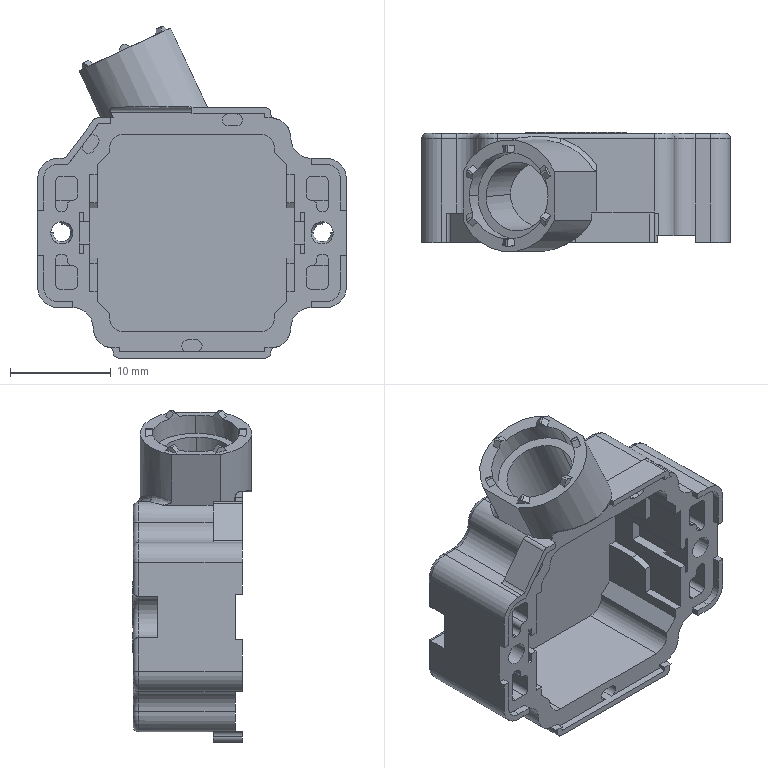Part | STEP file | _1-SO-416960001^MS1H1-40B30CB-A331Z_1_ASM_Motor mount assembly | 1 solid | 440 faces | box 30.6 x 11.855 x 32.912 mm | volume 2757 mm3 | plane 214 | cylinder 101 | spline 101 | torus 20 | cone 4 | commonest cylinder face diameters 1 x47 4 x12 1.2 x9 2.2 x8 10 x6 2.8 x4